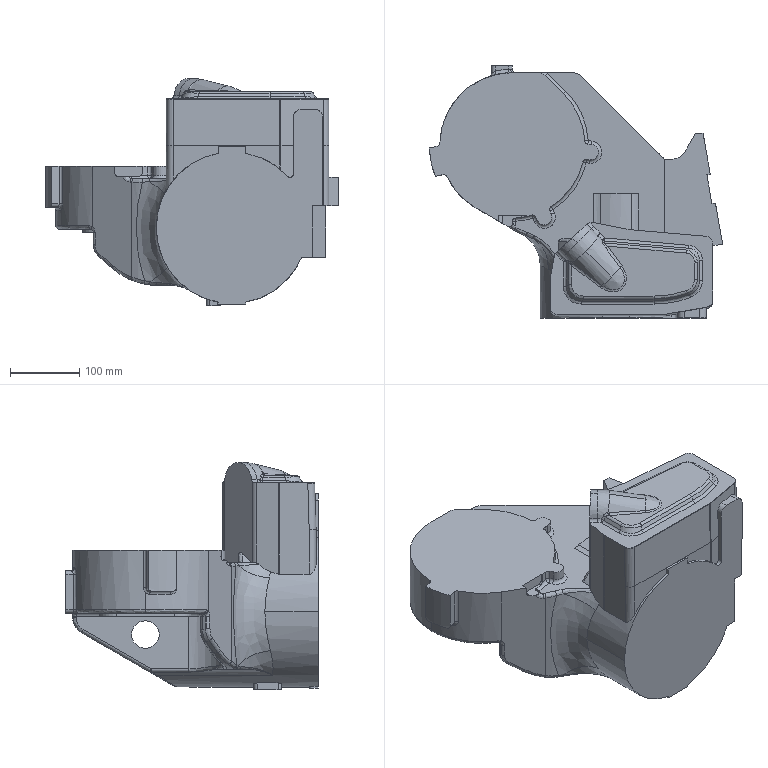Part | STEP file | Link3 | 1 solid | 342 faces | box 424.142 x 365 x 328.5 mm | volume 12864822 mm3 | cylinder 134 | plane 96 | spline 77 | cone 16 | torus 13 | sphere 6 | commonest cylinder face diameters 10 x56 6.8 x16 20 x13 40 x6 210 x5 48 x4